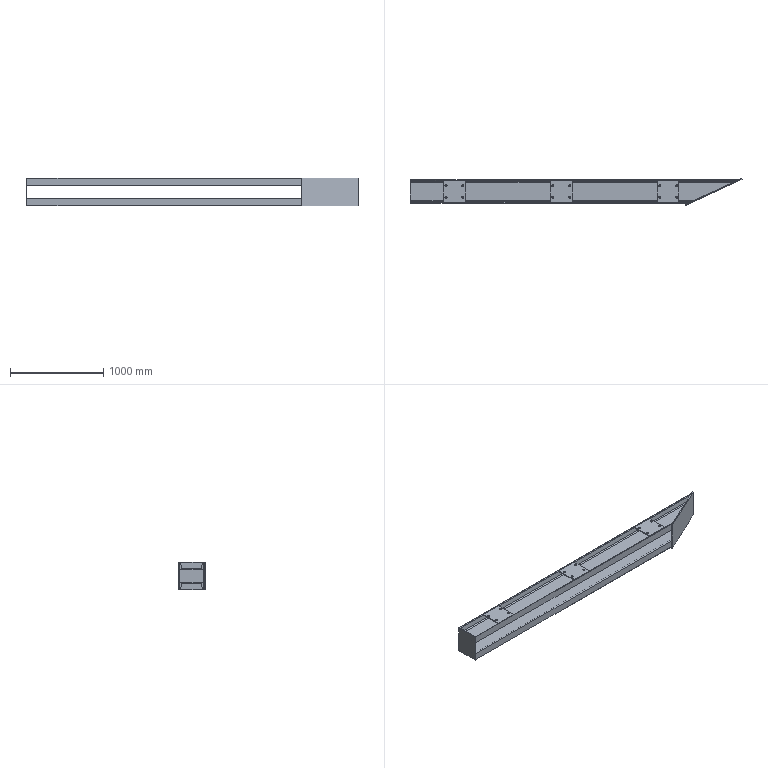Part | STEP file | Motor base support channel steel_Default<As machined> | 7 solids | 82 faces | box 3569 x 291.917 x 300 mm | volume 27407962 mm3 | plane 50 | cylinder 32 | commonest cylinder face diameters 22 x24 12 x4 24 x4